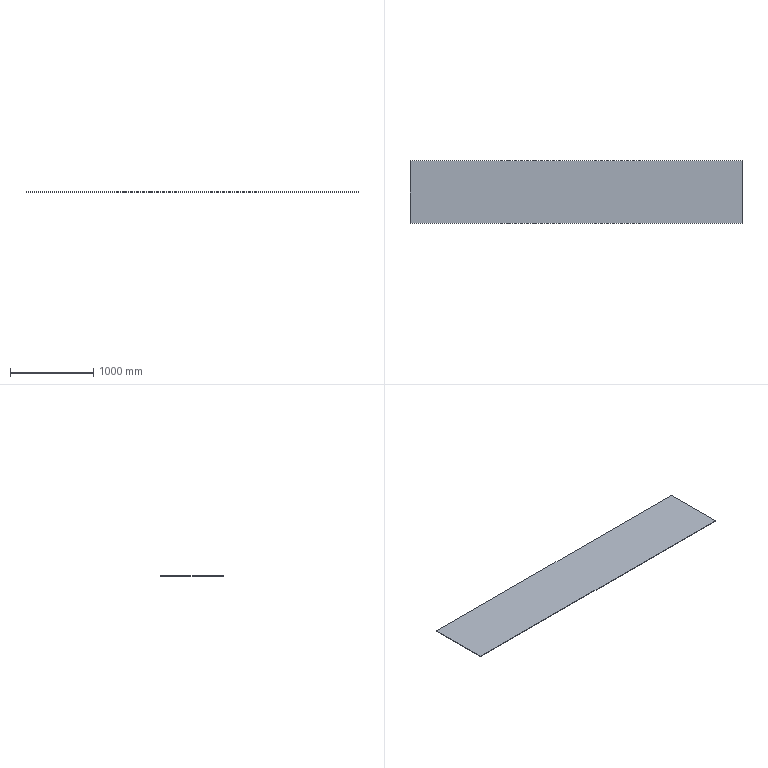Part | SolidWorks | features FlatPattern 1, SMBaseFlange 1, SheetMetal 1 | 1 solid | 6 faces | box 4000 x 750 x 6 mm | volume 18000000 mm3 | plane 6
STEP:
#1=CARTESIAN_POINT('',(-2000.,375.,0.));
#2=VERTEX_POINT('',#1);
#3=CARTESIAN_POINT('',(-2000.,-375.,0.));
#4=VERTEX_POINT('',#3);
#5=CARTESIAN_POINT('',(-2000.,-375.,0.));
#6=DIRECTION('',(0.,-1.,0.));
#7=VECTOR('',#6,1000.);
#8=LINE('',#5,#7);
#9=EDGE_CURVE('',#2,#4,#8,.T.);
#10=ORIENTED_EDGE('',*,*,#9,.F.);
#11=CARTESIAN_POINT('',(-2000.,375.,-6.));
#12=VERTEX_POINT('',#11);
#13=CARTESIAN_POINT('',(-2000.,375.,-6.));
#14=DIRECTION('',(0.,0.,1.));
#15=VECTOR('',#14,1000.);
#16=LINE('',#13,#15);
#17=EDGE_CURVE('',#12,#2,#16,.T.);
#18=ORIENTED_EDGE('',*,*,#17,.F.);
#19=CARTESIAN_POINT('',(-2000.,-375.,-6.));
#20=VERTEX_POINT('',#19);
#21=CARTESIAN_POINT('',(-2000.,-375.,-6.));
#22=DIRECTION('',(0.,-1.,0.));
#23=VECTOR('',#22,1000.);
#24=LINE('',#21,#23);
#25=EDGE_CURVE('',#12,#20,#24,.T.);
#26=ORIENTED_EDGE('',*,*,#25,.T.);
#27=CARTESIAN_POINT('',(-2000.,-375.,-6.));
#28=DIRECTION('',(0.,0.,1.));
#29=VECTOR('',#28,1000.);
#30=LINE('',#27,#29);
#31=EDGE_CURVE('',#20,#4,#30,.T.);
#32=ORIENTED_EDGE('',*,*,#31,.T.);
#33=EDGE_LOOP('',(#10,#18,#26,#32));
#34=FACE_OUTER_BOUND('',#33,.T.);
#35=CARTESIAN_POINT('',(-2000.,-375.,-6.));
#36=DIRECTION('',(-1.,0.,0.));
#37=DIRECTION('',(0.,0.,1.));
#38=AXIS2_PLACEMENT_3D('',#35,#36,#37);
#39=PLANE('',#38);
#40=ADVANCED_FACE('',(#34),#39,.T.);
#41=CARTESIAN_POINT('',(2000.,375.,0.));
#42=VERTEX_POINT('',#41);
#43=CARTESIAN_POINT('',(2000.,375.,0.));
#44=DIRECTION('',(-1.,0.,0.));
#45=VECTOR('',#44,1000.);
#46=LINE('',#43,#45);
#47=EDGE_CURVE('',#42,#2,#46,.T.);
#48=ORIENTED_EDGE('',*,*,#47,.F.);
#49=CARTESIAN_POINT('',(2000.,375.,-6.));
#50=VERTEX_POINT('',#49);
#51=CARTESIAN_POINT('',(2000.,375.,-6.));
#52=DIRECTION('',(0.,0.,1.));
#53=VECTOR('',#52,1000.);
#54=LINE('',#51,#53);
#55=EDGE_CURVE('',#50,#42,#54,.T.);
#56=ORIENTED_EDGE('',*,*,#55,.F.);
#57=CARTESIAN_POINT('',(2000.,375.,-6.));
#58=DIRECTION('',(-1.,0.,0.));
#59=VECTOR('',#58,1000.);
#60=LINE('',#57,#59);
#61=EDGE_CURVE('',#50,#12,#60,.T.);
#62=ORIENTED_EDGE('',*,*,#61,.T.);
#63=ORIENTED_EDGE('',*,*,#17,.T.);
#64=EDGE_LOOP('',(#48,#56,#62,#63));
#65=FACE_OUTER_BOUND('',#64,.T.);
#66=CARTESIAN_POINT('',(2000.,375.,-6.));
#67=DIRECTION('',(0.,1.,0.));
#68=DIRECTION('',(-1.,0.,0.));
#69=AXIS2_PLACEMENT_3D('',#66,#67,#68);
#70=PLANE('',#69);
#71=ADVANCED_FACE('',(#65),#70,.T.);
#72=CARTESIAN_POINT('',(2000.,-375.,0.));
#73=VERTEX_POINT('',#72);
#74=CARTESIAN_POINT('',(2000.,-375.,0.));
#75=DIRECTION('',(0.,1.,0.));
#76=VECTOR('',#75,1000.);
#77=LINE('',#74,#76);
#78=EDGE_CURVE('',#73,#42,#77,.T.);
#79=ORIENTED_EDGE('',*,*,#78,.F.);
#80=CARTESIAN_POINT('',(2000.,-375.,-6.));
#81=VERTEX_POINT('',#80);
#82=CARTESIAN_POINT('',(2000.,-375.,-6.));
#83=DIRECTION('',(0.,0.,1.));
#84=VECTOR('',#83,1000.);
#85=LINE('',#82,#84);
#86=EDGE_CURVE('',#81,#73,#85,.T.);
#87=ORIENTED_EDGE('',*,*,#86,.F.);
#88=CARTESIAN_POINT('',(2000.,-375.,-6.));
#89=DIRECTION('',(0.,1.,0.));
#90=VECTOR('',#89,1000.);
#91=LINE('',#88,#90);
#92=EDGE_CURVE('',#81,#50,#91,.T.);
#93=ORIENTED_EDGE('',*,*,#92,.T.);
#94=ORIENTED_EDGE('',*,*,#55,.T.);
#95=EDGE_LOOP('',(#79,#87,#93,#94));
#96=FACE_OUTER_BOUND('',#95,.T.);
#97=CARTESIAN_POINT('',(2000.,-375.,-6.));
#98=DIRECTION('',(1.,0.,0.));
#99=DIRECTION('',(0.,0.,-1.));
#100=AXIS2_PLACEMENT_3D('',#97,#98,#99);
#101=PLANE('',#100);
#102=ADVANCED_FACE('',(#96),#101,.T.);
#103=CARTESIAN_POINT('',(2000.,-375.,0.));
#104=DIRECTION('',(1.,0.,0.));
#105=VECTOR('',#104,1000.);
#106=LINE('',#103,#105);
#107=EDGE_CURVE('',#4,#73,#106,.T.);
#108=ORIENTED_EDGE('',*,*,#107,.F.);
#109=ORIENTED_EDGE('',*,*,#31,.F.);
#110=CARTESIAN_POINT('',(2000.,-375.,-6.));
#111=DIRECTION('',(1.,0.,0.));
#112=VECTOR('',#111,1000.);
#113=LINE('',#110,#112);
#114=EDGE_CURVE('',#20,#81,#113,.T.);
#115=ORIENTED_EDGE('',*,*,#114,.T.);
#116=ORIENTED_EDGE('',*,*,#86,.T.);
#117=EDGE_LOOP('',(#108,#109,#115,#116));
#118=FACE_OUTER_BOUND('',#117,.T.);
#119=CARTESIAN_POINT('',(2000.,-375.,-6.));
#120=DIRECTION('',(0.,-1.,0.));
#121=DIRECTION('',(1.,0.,0.));
#122=AXIS2_PLACEMENT_3D('',#119,#120,#121);
#123=PLANE('',#122);
#124=ADVANCED_FACE('',(#118),#123,.T.);
#125=ORIENTED_EDGE('',*,*,#25,.F.);
#126=ORIENTED_EDGE('',*,*,#61,.F.);
#127=ORIENTED_EDGE('',*,*,#92,.F.);
#128=ORIENTED_EDGE('',*,*,#114,.F.);
#129=EDGE_LOOP('',(#125,#126,#127,#128));
#130=FACE_OUTER_BOUND('',#129,.T.);
#131=CARTESIAN_POINT('',(0.,0.,-6.));
#132=DIRECTION('',(0.,0.,1.));
#133=DIRECTION('',(1.,0.,0.));
#134=AXIS2_PLACEMENT_3D('',#131,#132,#133);
#135=PLANE('',#134);
#136=ADVANCED_FACE('',(#130),#135,.F.);
#137=ORIENTED_EDGE('',*,*,#9,.T.);
#138=ORIENTED_EDGE('',*,*,#107,.T.);
#139=ORIENTED_EDGE('',*,*,#78,.T.);
#140=ORIENTED_EDGE('',*,*,#47,.T.);
#141=EDGE_LOOP('',(#137,#138,#139,#140));
#142=FACE_OUTER_BOUND('',#141,.T.);
#143=CARTESIAN_POINT('',(0.,0.,0.));
#144=DIRECTION('',(0.,0.,1.));
#145=DIRECTION('',(1.,0.,0.));
#146=AXIS2_PLACEMENT_3D('',#143,#144,#145);
#147=PLANE('',#146);
#148=ADVANCED_FACE('',(#142),#147,.T.);
#149=CLOSED_SHELL('',(#40,#71,#102,#124,#136,#148));
#150=MANIFOLD_SOLID_BREP('',#149);
#151=CARTESIAN_POINT('',(0.,0.,0.));
#152=DIRECTION('',(0.,0.,1.));
#153=DIRECTION('',(1.,0.,0.));
#154=AXIS2_PLACEMENT_3D('',#151,#152,#153);
#155=(LENGTH_UNIT()NAMED_UNIT(*)SI_UNIT(.MILLI.,.METRE.));
#156=UNCERTAINTY_MEASURE_WITH_UNIT(LENGTH_MEASURE(0.00001),#155,'','');
#157=(NAMED_UNIT(*)PLANE_ANGLE_UNIT()SI_UNIT($,.RADIAN.));
#158=(NAMED_UNIT(*)SI_UNIT($,.STERADIAN.)SOLID_ANGLE_UNIT());
#159=(GEOMETRIC_REPRESENTATION_CONTEXT(3)GLOBAL_UNCERTAINTY_ASSIGNED_CONTEXT((#156))GLOBAL_UNIT_ASSIGNED_CONTEXT((#155,#157,#158))REPRESENTATION_CONTEXT('',''));
#160=ADVANCED_BREP_SHAPE_REPRESENTATION('',(#150,#154),#159);